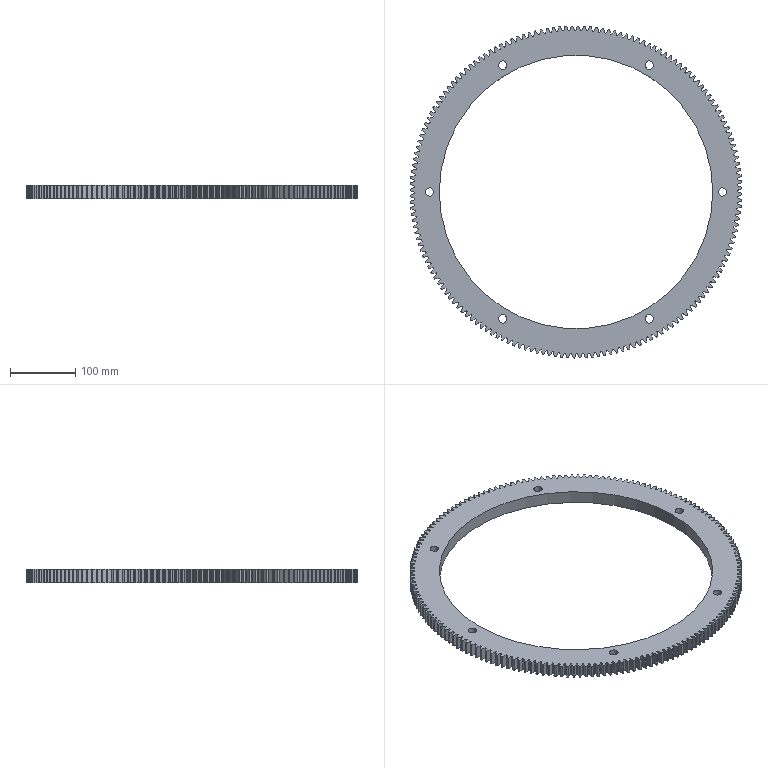Part | SolidWorks | features ICE 2, CirPattern 1, Extrusion 1, HoleWzd 1 | 1 solid | 688 faces | box 509.982 x 509.982 x 20 mm | volume 1197057 mm3 | cylinder 350 | spline 336 | plane 2 | commonest cylinder face diameters 496.5 x168 510 x168 13 x12 420 x2